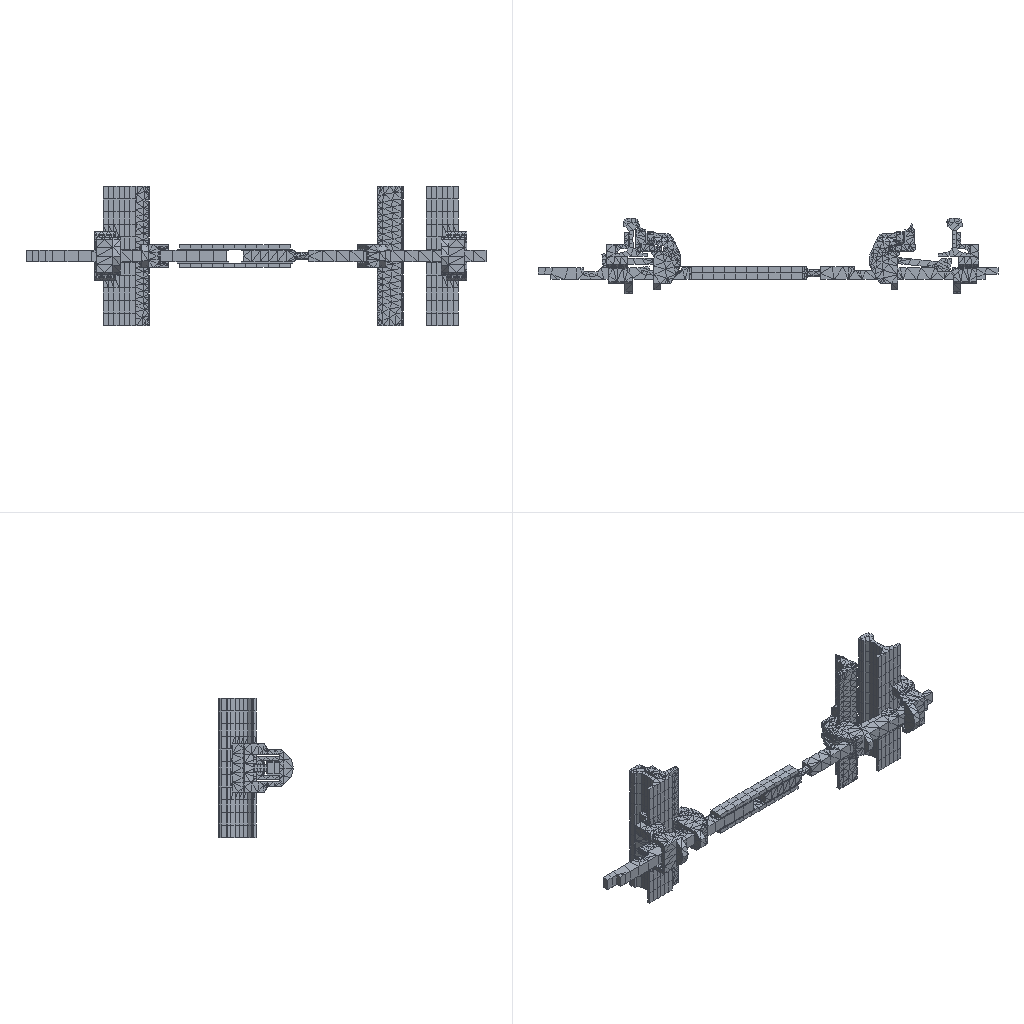Simulation study | ansys workbench
Set-up summary, first 288 of 305 lines:
category,name,step,type,value,unit,region
solver,ansys_mapdl
solver,version,,,22.1
solver,version,,,22.1
solver,version,,,22.1
solver,version,,,22.1
solver,version,,,22.1
solver,version,,,22.1
solver,version,,,22.1
units,MPA,,stated
analysis,deck1,,static,static
load_step,requested,,,1
analysis,nlgeom,,,False
mesh,nodes,,,34125
mesh,elements,,,18517
element_type,ANSYS 186 (type 1),,solid,308
element_type,ANSYS 186 (type 2),,solid,308
element_type,ANSYS 187 (type 3),,solid,2347
element_type,ANSYS 187 (type 4),,solid,2347
element_type,ANSYS 187 (type 5),,solid,1336
element_type,ANSYS 187 (type 6),,solid,1336
element_type,ANSYS 186 (type 7),,solid,16
element_type,ANSYS 186 (type 8),,solid,16
element_type,ANSYS 186 (type 9),,solid,148
element_type,ANSYS 186 (type 10),,solid,148
element_type,ANSYS 186 (type 11),,solid,20
element_type,ANSYS 186 (type 12),,solid,20
element_type,ANSYS 186 (type 13),,solid,16
element_type,ANSYS 186 (type 14),,solid,16
element_type,ANSYS 186 (type 15),,solid,16
element_type,ANSYS 186 (type 16),,solid,16
element_type,ANSYS 187 (type 17),,solid,423
element_type,ANSYS 187 (type 18),,solid,506
element_type,ANSYS 186 (type 19),,solid,59
element_type,ANSYS 187 (type 20),,solid,2674
element_type,ANSYS 187 (type 21),,solid,2475
element_type,ANSYS 174 (type 22),,contact,226
element_type,ANSYS 170 (type 23),,target,226
element_type,ANSYS 174 (type 24),,contact,129
element_type,ANSYS 170 (type 25),,target,129
element_type,ANSYS 174 (type 26),,contact,129
element_type,ANSYS 170 (type 27),,target,129
element_type,ANSYS 174 (type 28),,contact,57
element_type,ANSYS 170 (type 29),,target,57
element_type,ANSYS 174 (type 30),,contact,126
element_type,ANSYS 170 (type 31),,target,126
element_type,ANSYS 174 (type 32),,contact,57
element_type,ANSYS 170 (type 33),,target,57
element_type,ANSYS 174 (type 34),,contact,224
element_type,ANSYS 170 (type 35),,target,224
element_type,ANSYS 174 (type 36),,contact,37
element_type,ANSYS 170 (type 37),,target,37
element_type,ANSYS 174 (type 38),,contact,9
element_type,ANSYS 170 (type 39),,target,9
element_type,ANSYS 174 (type 40),,contact,34
element_type,ANSYS 170 (type 41),,target,34
element_type,ANSYS 174 (type 42),,contact,54
element_type,ANSYS 170 (type 43),,target,54
element_type,ANSYS 174 (type 44),,contact,32
element_type,ANSYS 170 (type 45),,target,32
element_type,ANSYS 174 (type 46),,contact,12
element_type,ANSYS 170 (type 47),,target,12
element_type,ANSYS 174 (type 48),,contact,217
element_type,ANSYS 170 (type 49),,target,217
element_type,ANSYS 174 (type 50),,contact,48
element_type,ANSYS 170 (type 51),,target,48
element_type,ANSYS 174 (type 52),,contact,207
element_type,ANSYS 170 (type 53),,target,207
element_type,ANSYS 174 (type 54),,contact,26
element_type,ANSYS 170 (type 55),,target,26
element_type,ANSYS 174 (type 56),,contact,26
element_type,ANSYS 170 (type 57),,target,26
element_type,ANSYS 174 (type 58),,contact,26
element_type,ANSYS 170 (type 59),,target,26
element_type,ANSYS 174 (type 60),,contact,14
element_type,ANSYS 170 (type 61),,target,14
element_type,ANSYS 174 (type 62),,contact,26
element_type,ANSYS 170 (type 63),,target,26
element_type,ANSYS 174 (type 64),,contact,26
element_type,ANSYS 170 (type 65),,target,26
element_type,ANSYS 174 (type 66),,contact,26
element_type,ANSYS 170 (type 67),,target,26
element_type,ANSYS 174 (type 68),,contact,14
element_type,ANSYS 170 (type 69),,target,14
element_type,ANSYS 174 (type 70),,contact,22
element_type,ANSYS 170 (type 71),,target,22
element_type,ANSYS 174 (type 72),,contact,22
element_type,ANSYS 170 (type 73),,target,22
element_type,ANSYS 174 (type 74),,contact,32
element_type,ANSYS 170 (type 75),,target,32
element_type,ANSYS 174 (type 76),,contact,32
element_type,ANSYS 170 (type 77),,target,32
element_type,ANSYS 174 (type 78),,contact,71
element_type,ANSYS 170 (type 79),,target,71
element_type,ANSYS 154 (type 80),,surface,44
load,load commands in deck,,count,3
bc,support commands in deck,,count,1
named_set,_FIXEDSU,,component
analysis,deck2,,modal,HARM; modal
load_step,requested,,,3
analysis,nlgeom,,,False
mesh,nodes,,,0
mesh,elements,,,0
load,load commands in deck,,count,3
bc,support commands in deck,,count,0
named_set,_CM197_1,,component
named_set,_CM197_2,,component
named_set,_CM197_4,,component
analysis,deck3,,modal,modal
load_step,requested,,,1
analysis,nlgeom,,,False
mesh,nodes,,,34119
mesh,elements,,,18465
element_type,ANSYS 186 (type 1),,solid,308
element_type,ANSYS 186 (type 2),,solid,308
element_type,ANSYS 187 (type 3),,solid,2344
element_type,ANSYS 187 (type 4),,solid,2344
element_type,ANSYS 187 (type 5),,solid,1336
element_type,ANSYS 187 (type 6),,solid,1336
element_type,ANSYS 186 (type 7),,solid,16
element_type,ANSYS 186 (type 8),,solid,16
element_type,ANSYS 186 (type 9),,solid,148
element_type,ANSYS 186 (type 10),,solid,148
element_type,ANSYS 186 (type 11),,solid,20
element_type,ANSYS 186 (type 12),,solid,20
element_type,ANSYS 186 (type 13),,solid,16
element_type,ANSYS 186 (type 14),,solid,16
element_type,ANSYS 186 (type 15),,solid,16
element_type,ANSYS 186 (type 16),,solid,16
element_type,ANSYS 187 (type 17),,solid,423
element_type,ANSYS 187 (type 18),,solid,506
element_type,ANSYS 186 (type 19),,solid,59
element_type,ANSYS 187 (type 20),,solid,2674
element_type,ANSYS 187 (type 21),,solid,2475
element_type,ANSYS 174 (type 22),,contact,225
element_type,ANSYS 170 (type 23),,target,225
element_type,ANSYS 174 (type 24),,contact,129
element_type,ANSYS 170 (type 25),,target,129
element_type,ANSYS 174 (type 26),,contact,129
element_type,ANSYS 170 (type 27),,target,129
element_type,ANSYS 174 (type 28),,contact,57
element_type,ANSYS 170 (type 29),,target,57
element_type,ANSYS 174 (type 30),,contact,126
element_type,ANSYS 170 (type 31),,target,126
element_type,ANSYS 174 (type 32),,contact,57
element_type,ANSYS 170 (type 33),,target,57
element_type,ANSYS 174 (type 34),,contact,224
element_type,ANSYS 170 (type 35),,target,224
element_type,ANSYS 174 (type 36),,contact,37
element_type,ANSYS 170 (type 37),,target,37
element_type,ANSYS 174 (type 38),,contact,9
element_type,ANSYS 170 (type 39),,target,9
element_type,ANSYS 174 (type 40),,contact,34
element_type,ANSYS 170 (type 41),,target,34
element_type,ANSYS 174 (type 42),,contact,54
element_type,ANSYS 170 (type 43),,target,54
element_type,ANSYS 174 (type 44),,contact,32
element_type,ANSYS 170 (type 45),,target,32
element_type,ANSYS 174 (type 46),,contact,12
element_type,ANSYS 170 (type 47),,target,12
element_type,ANSYS 174 (type 48),,contact,217
element_type,ANSYS 170 (type 49),,target,217
element_type,ANSYS 174 (type 50),,contact,48
element_type,ANSYS 170 (type 51),,target,48
element_type,ANSYS 174 (type 52),,contact,207
element_type,ANSYS 170 (type 53),,target,207
element_type,ANSYS 174 (type 54),,contact,26
element_type,ANSYS 170 (type 55),,target,26
element_type,ANSYS 174 (type 56),,contact,26
element_type,ANSYS 170 (type 57),,target,26
element_type,ANSYS 174 (type 58),,contact,26
element_type,ANSYS 170 (type 59),,target,26
element_type,ANSYS 174 (type 60),,contact,14
element_type,ANSYS 170 (type 61),,target,14
element_type,ANSYS 174 (type 62),,contact,26
element_type,ANSYS 170 (type 63),,target,26
element_type,ANSYS 174 (type 64),,contact,26
element_type,ANSYS 170 (type 65),,target,26
element_type,ANSYS 174 (type 66),,contact,26
element_type,ANSYS 170 (type 67),,target,26
element_type,ANSYS 174 (type 68),,contact,14
element_type,ANSYS 170 (type 69),,target,14
element_type,ANSYS 174 (type 70),,contact,22
element_type,ANSYS 170 (type 71),,target,22
element_type,ANSYS 174 (type 72),,contact,22
element_type,ANSYS 170 (type 73),,target,22
element_type,ANSYS 174 (type 74),,contact,32
element_type,ANSYS 170 (type 75),,target,32
element_type,ANSYS 174 (type 76),,contact,32
element_type,ANSYS 170 (type 77),,target,32
element_type,ANSYS 174 (type 78),,contact,71
element_type,ANSYS 170 (type 79),,target,71
load,load commands in deck,,count,0
bc,support commands in deck,,count,0
named_set,_CONSTRAINEDNODES,,component
material,3,,in results
material,4,,in results
material,11,,in results
material,12,,in results
material,19,,in results
material,20,,in results
material,21,,in results
material,1,,in results
material,2,,in results
material,5,,in results
material,6,,in results
material,7,,in results
material,8,,in results
material,9,,in results
material,10,,in results
material,13,,in results
material,14,,in results
material,15,,in results
material,16,,in results
material,17,,in results
material,18,,in results
material,20,,in results
material,1,,in results
material,2,,in results
material,3,,in results
material,4,,in results
material,5,,in results
material,6,,in results
material,7,,in results
material,8,,in results
material,9,,in results
material,10,,in results
material,11,,in results
material,12,,in results
material,13,,in results
material,14,,in results
material,15,,in results
material,16,,in results
material,17,,in results
material,18,,in results
material,19,,in results
material,20,,in results
material,21,,in results
material,1,,in results
material,2,,in results
material,3,,in results
material,4,,in results
material,5,,in results
material,6,,in results
material,7,,in results
material,8,,in results
material,9,,in results
material,10,,in results
material,11,,in results
material,12,,in results
material,13,,in results
material,14,,in results
material,15,,in results
material,16,,in results
material,17,,in results
material,18,,in results
material,19,,in results
material,20,,in results
material,21,,in results
material,1,,in results
material,3,,in results
material,4,,in results
material,6,,in results
material,7,,in results
material,8,,in results
material,9,,in results
material,10,,in results
material,11,,in results
material,12,,in results
material,13,,in results
material,14,,in results
material,15,,in results
material,16,,in results
material,17,,in results
material,18,,in results
material,19,,in results
material,2,,in results
material,5,,in results
material,18,,in results
material,20,,in results
material,21,,in results
material,1,,in results
material,2,,in results
material,3,,in results
material,4,,in results
material,5,,in results
material,6,,in results
material,7,,in results
Results summary:
result,analysis,,,static
result,last_loadstep,,,1
result,primary field,,,displacement
result,reaction total,1,FX,-723.357,N
result,reaction total,1,FY,3270.222,N
result,reaction total,1,FZ,-6.936,N
result,mass,,,0.1125,"NMM: mm, ton, N, s, mV, mA, degC"
result,analysis,,,static
result,last_loadstep,,,1
result,primary field,,,displacement
result,reaction total,1,FX,723.355,N
result,reaction total,1,FY,46729.778,N
result,reaction total,1,FZ,6.937,N
result,mass,,,0.1615,"NMM: mm, ton, N, s, mV, mA, degC"
result,analysis,,,static
result,last_loadstep,,,1
result,primary field,,,displacement
result,reaction total,1,FX,-0.001237,N
result,reaction total,1,FY,50000,N
result,reaction total,1,FZ,0.000294,N
result,mass,,,0.2741,"NMM: mm, ton, N, s, mV, mA, degC"
result,analysis,,,msup
result,last_loadstep,,,1
result,primary field,,,displacement
result,mass,,,0.2741,"NMM: mm, ton, N, s, mV, mA, degC"
result,analysis,,,modal
result,last_loadstep,,,1
result,primary field,,,displacement
result,analysis,,,modal
result,last_loadstep,,,1
result,primary field,,,displacement
result,analysis,,,modal
result,last_loadstep,,,1
result,primary field,,,displacement